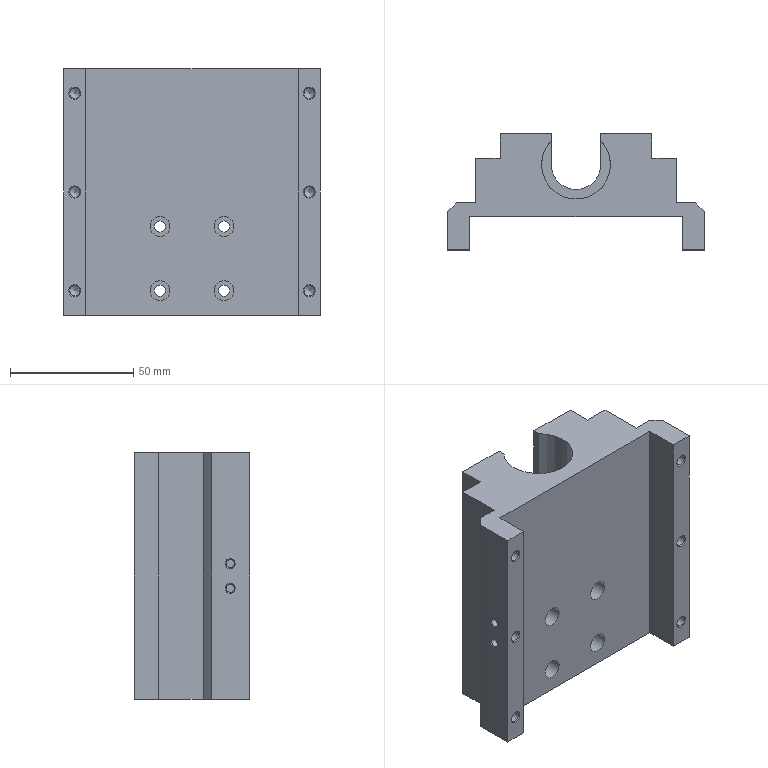Part | NX | 1 solid | 72 faces | box 104 x 47 x 100 mm | volume 229992 mm3 | plane 36 | cylinder 20 | cone 16 | commonest cylinder face diameters 4.2 x6 8 x6 4.5 x4 3.3 x2 20 x1 28 x1